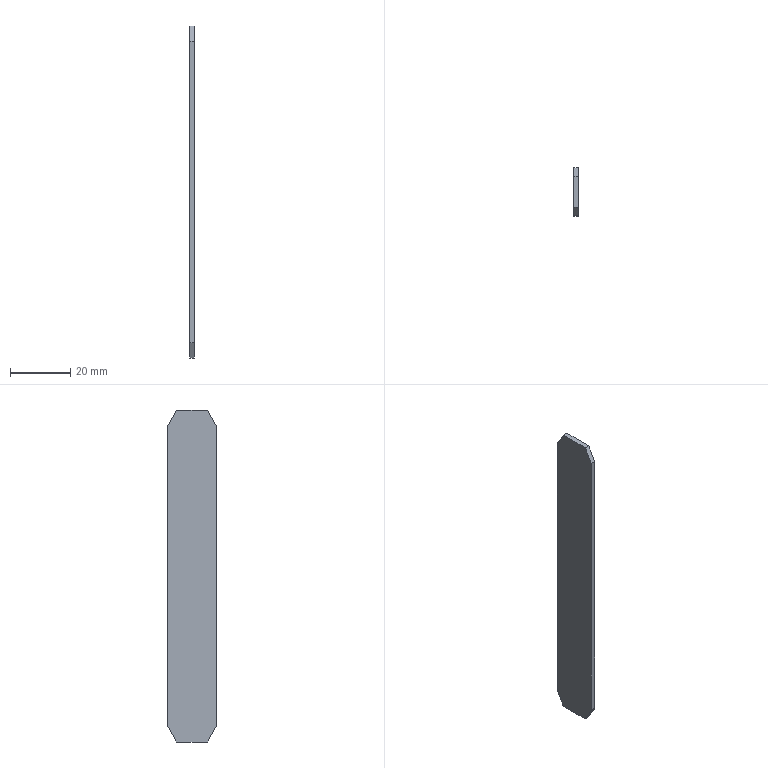Part | STEP file | 11-FG-B03111 | 1 solid | 10 faces | box 1.6 x 16 x 110 mm | volume 2770 mm3 | plane 10
STEP:
#1=CARTESIAN_POINT('',(0.8,-8.,105.));
#2=VERTEX_POINT('',#1);
#3=CARTESIAN_POINT('',(0.8,-8.,5.));
#4=VERTEX_POINT('',#3);
#5=CARTESIAN_POINT('',(0.8,-8.,110.));
#6=DIRECTION('',(0.,0.,-1.));
#7=VECTOR('',#6,1000.);
#8=LINE('',#5,#7);
#9=EDGE_CURVE('',#2,#4,#8,.T.);
#10=ORIENTED_EDGE('',*,*,#9,.T.);
#11=CARTESIAN_POINT('',(0.8,-5.113,0.));
#12=VERTEX_POINT('',#11);
#13=CARTESIAN_POINT('',(0.8,-8.,5.));
#14=DIRECTION('',(0.,0.5,-0.866));
#15=VECTOR('',#14,1000.);
#16=LINE('',#13,#15);
#17=EDGE_CURVE('',#4,#12,#16,.T.);
#18=ORIENTED_EDGE('',*,*,#17,.T.);
#19=CARTESIAN_POINT('',(0.8,5.113,0.));
#20=VERTEX_POINT('',#19);
#21=CARTESIAN_POINT('',(0.8,8.,0.));
#22=DIRECTION('',(0.,1.,0.));
#23=VECTOR('',#22,1000.);
#24=LINE('',#21,#23);
#25=EDGE_CURVE('',#12,#20,#24,.T.);
#26=ORIENTED_EDGE('',*,*,#25,.T.);
#27=CARTESIAN_POINT('',(0.8,8.,5.));
#28=VERTEX_POINT('',#27);
#29=CARTESIAN_POINT('',(0.8,8.,5.));
#30=DIRECTION('',(0.,0.5,0.866));
#31=VECTOR('',#30,1000.);
#32=LINE('',#29,#31);
#33=EDGE_CURVE('',#20,#28,#32,.T.);
#34=ORIENTED_EDGE('',*,*,#33,.T.);
#35=CARTESIAN_POINT('',(0.8,8.,105.));
#36=VERTEX_POINT('',#35);
#37=CARTESIAN_POINT('',(0.8,8.,110.));
#38=DIRECTION('',(0.,0.,-1.));
#39=VECTOR('',#38,1000.);
#40=LINE('',#37,#39);
#41=EDGE_CURVE('',#36,#28,#40,.T.);
#42=ORIENTED_EDGE('',*,*,#41,.F.);
#43=CARTESIAN_POINT('',(0.8,5.113,110.));
#44=VERTEX_POINT('',#43);
#45=CARTESIAN_POINT('',(0.8,5.113,110.));
#46=DIRECTION('',(0.,-0.5,0.866));
#47=VECTOR('',#46,1000.);
#48=LINE('',#45,#47);
#49=EDGE_CURVE('',#36,#44,#48,.T.);
#50=ORIENTED_EDGE('',*,*,#49,.T.);
#51=CARTESIAN_POINT('',(0.8,-5.113,110.));
#52=VERTEX_POINT('',#51);
#53=CARTESIAN_POINT('',(0.8,8.,110.));
#54=DIRECTION('',(0.,1.,0.));
#55=VECTOR('',#54,1000.);
#56=LINE('',#53,#55);
#57=EDGE_CURVE('',#52,#44,#56,.T.);
#58=ORIENTED_EDGE('',*,*,#57,.F.);
#59=CARTESIAN_POINT('',(0.8,-5.113,110.));
#60=DIRECTION('',(0.,-0.5,-0.866));
#61=VECTOR('',#60,1000.);
#62=LINE('',#59,#61);
#63=EDGE_CURVE('',#52,#2,#62,.T.);
#64=ORIENTED_EDGE('',*,*,#63,.T.);
#65=EDGE_LOOP('',(#10,#18,#26,#34,#42,#50,#58,#64));
#66=FACE_OUTER_BOUND('',#65,.T.);
#67=CARTESIAN_POINT('',(0.8,8.,110.));
#68=DIRECTION('',(-1.,0.,0.));
#69=DIRECTION('',(0.,-1.,0.));
#70=AXIS2_PLACEMENT_3D('',#67,#68,#69);
#71=PLANE('',#70);
#72=ADVANCED_FACE('',(#66),#71,.F.);
#73=ORIENTED_EDGE('',*,*,#41,.T.);
#74=CARTESIAN_POINT('',(-0.8,8.,5.));
#75=VERTEX_POINT('',#74);
#76=CARTESIAN_POINT('',(-0.8,8.,5.));
#77=DIRECTION('',(-1.,0.,0.));
#78=VECTOR('',#77,1000.);
#79=LINE('',#76,#78);
#80=EDGE_CURVE('',#28,#75,#79,.T.);
#81=ORIENTED_EDGE('',*,*,#80,.T.);
#82=CARTESIAN_POINT('',(-0.8,8.,105.));
#83=VERTEX_POINT('',#82);
#84=CARTESIAN_POINT('',(-0.8,8.,110.));
#85=DIRECTION('',(0.,0.,-1.));
#86=VECTOR('',#85,1000.);
#87=LINE('',#84,#86);
#88=EDGE_CURVE('',#83,#75,#87,.T.);
#89=ORIENTED_EDGE('',*,*,#88,.F.);
#90=CARTESIAN_POINT('',(0.8,8.,105.));
#91=DIRECTION('',(1.,0.,0.));
#92=VECTOR('',#91,1000.);
#93=LINE('',#90,#92);
#94=EDGE_CURVE('',#83,#36,#93,.T.);
#95=ORIENTED_EDGE('',*,*,#94,.T.);
#96=EDGE_LOOP('',(#73,#81,#89,#95));
#97=FACE_OUTER_BOUND('',#96,.T.);
#98=CARTESIAN_POINT('',(-0.8,8.,110.));
#99=DIRECTION('',(0.,-1.,0.));
#100=DIRECTION('',(0.,0.,-1.));
#101=AXIS2_PLACEMENT_3D('',#98,#99,#100);
#102=PLANE('',#101);
#103=ADVANCED_FACE('',(#97),#102,.F.);
#104=CARTESIAN_POINT('',(-0.8,5.113,0.));
#105=VERTEX_POINT('',#104);
#106=CARTESIAN_POINT('',(-0.8,-5.113,0.));
#107=VERTEX_POINT('',#106);
#108=CARTESIAN_POINT('',(-0.8,8.,0.));
#109=DIRECTION('',(0.,-1.,0.));
#110=VECTOR('',#109,1000.);
#111=LINE('',#108,#110);
#112=EDGE_CURVE('',#105,#107,#111,.T.);
#113=ORIENTED_EDGE('',*,*,#112,.T.);
#114=CARTESIAN_POINT('',(-0.8,-8.,5.));
#115=VERTEX_POINT('',#114);
#116=CARTESIAN_POINT('',(-0.8,-8.,5.));
#117=DIRECTION('',(0.,-0.5,0.866));
#118=VECTOR('',#117,1000.);
#119=LINE('',#116,#118);
#120=EDGE_CURVE('',#107,#115,#119,.T.);
#121=ORIENTED_EDGE('',*,*,#120,.T.);
#122=CARTESIAN_POINT('',(-0.8,-8.,105.));
#123=VERTEX_POINT('',#122);
#124=CARTESIAN_POINT('',(-0.8,-8.,110.));
#125=DIRECTION('',(0.,0.,-1.));
#126=VECTOR('',#125,1000.);
#127=LINE('',#124,#126);
#128=EDGE_CURVE('',#123,#115,#127,.T.);
#129=ORIENTED_EDGE('',*,*,#128,.F.);
#130=CARTESIAN_POINT('',(-0.8,-5.113,110.));
#131=VERTEX_POINT('',#130);
#132=CARTESIAN_POINT('',(-0.8,-5.113,110.));
#133=DIRECTION('',(0.,0.5,0.866));
#134=VECTOR('',#133,1000.);
#135=LINE('',#132,#134);
#136=EDGE_CURVE('',#123,#131,#135,.T.);
#137=ORIENTED_EDGE('',*,*,#136,.T.);
#138=CARTESIAN_POINT('',(-0.8,5.113,110.));
#139=VERTEX_POINT('',#138);
#140=CARTESIAN_POINT('',(-0.8,8.,110.));
#141=DIRECTION('',(0.,-1.,0.));
#142=VECTOR('',#141,1000.);
#143=LINE('',#140,#142);
#144=EDGE_CURVE('',#139,#131,#143,.T.);
#145=ORIENTED_EDGE('',*,*,#144,.F.);
#146=CARTESIAN_POINT('',(-0.8,5.113,110.));
#147=DIRECTION('',(0.,0.5,-0.866));
#148=VECTOR('',#147,1000.);
#149=LINE('',#146,#148);
#150=EDGE_CURVE('',#139,#83,#149,.T.);
#151=ORIENTED_EDGE('',*,*,#150,.T.);
#152=ORIENTED_EDGE('',*,*,#88,.T.);
#153=CARTESIAN_POINT('',(-0.8,8.,5.));
#154=DIRECTION('',(0.,-0.5,-0.866));
#155=VECTOR('',#154,1000.);
#156=LINE('',#153,#155);
#157=EDGE_CURVE('',#75,#105,#156,.T.);
#158=ORIENTED_EDGE('',*,*,#157,.T.);
#159=EDGE_LOOP('',(#113,#121,#129,#137,#145,#151,#152,#158));
#160=FACE_OUTER_BOUND('',#159,.T.);
#161=CARTESIAN_POINT('',(-0.8,8.,110.));
#162=DIRECTION('',(1.,0.,0.));
#163=DIRECTION('',(0.,1.,0.));
#164=AXIS2_PLACEMENT_3D('',#161,#162,#163);
#165=PLANE('',#164);
#166=ADVANCED_FACE('',(#160),#165,.F.);
#167=ORIENTED_EDGE('',*,*,#128,.T.);
#168=CARTESIAN_POINT('',(-0.8,-8.,5.));
#169=DIRECTION('',(1.,0.,0.));
#170=VECTOR('',#169,1000.);
#171=LINE('',#168,#170);
#172=EDGE_CURVE('',#115,#4,#171,.T.);
#173=ORIENTED_EDGE('',*,*,#172,.T.);
#174=ORIENTED_EDGE('',*,*,#9,.F.);
#175=CARTESIAN_POINT('',(-0.8,-8.,105.));
#176=DIRECTION('',(-1.,0.,0.));
#177=VECTOR('',#176,1000.);
#178=LINE('',#175,#177);
#179=EDGE_CURVE('',#2,#123,#178,.T.);
#180=ORIENTED_EDGE('',*,*,#179,.T.);
#181=EDGE_LOOP('',(#167,#173,#174,#180));
#182=FACE_OUTER_BOUND('',#181,.T.);
#183=CARTESIAN_POINT('',(-0.8,-8.,110.));
#184=DIRECTION('',(0.,1.,0.));
#185=DIRECTION('',(0.,0.,1.));
#186=AXIS2_PLACEMENT_3D('',#183,#184,#185);
#187=PLANE('',#186);
#188=ADVANCED_FACE('',(#182),#187,.F.);
#189=ORIENTED_EDGE('',*,*,#144,.T.);
#190=CARTESIAN_POINT('',(0.8,-5.113,110.));
#191=DIRECTION('',(1.,0.,0.));
#192=VECTOR('',#191,1000.);
#193=LINE('',#190,#192);
#194=EDGE_CURVE('',#131,#52,#193,.T.);
#195=ORIENTED_EDGE('',*,*,#194,.T.);
#196=ORIENTED_EDGE('',*,*,#57,.T.);
#197=CARTESIAN_POINT('',(-0.8,5.113,110.));
#198=DIRECTION('',(-1.,0.,0.));
#199=VECTOR('',#198,1000.);
#200=LINE('',#197,#199);
#201=EDGE_CURVE('',#44,#139,#200,.T.);
#202=ORIENTED_EDGE('',*,*,#201,.T.);
#203=EDGE_LOOP('',(#189,#195,#196,#202));
#204=FACE_OUTER_BOUND('',#203,.T.);
#205=CARTESIAN_POINT('',(0.,0.,110.));
#206=DIRECTION('',(0.,0.,1.));
#207=DIRECTION('',(1.,0.,0.));
#208=AXIS2_PLACEMENT_3D('',#205,#206,#207);
#209=PLANE('',#208);
#210=ADVANCED_FACE('',(#204),#209,.T.);
#211=ORIENTED_EDGE('',*,*,#25,.F.);
#212=CARTESIAN_POINT('',(0.,-5.113,0.));
#213=DIRECTION('',(-1.,0.,0.));
#214=VECTOR('',#213,1000.);
#215=LINE('',#212,#214);
#216=EDGE_CURVE('',#12,#107,#215,.T.);
#217=ORIENTED_EDGE('',*,*,#216,.T.);
#218=ORIENTED_EDGE('',*,*,#112,.F.);
#219=CARTESIAN_POINT('',(0.,5.113,0.));
#220=DIRECTION('',(1.,0.,0.));
#221=VECTOR('',#220,1000.);
#222=LINE('',#219,#221);
#223=EDGE_CURVE('',#105,#20,#222,.T.);
#224=ORIENTED_EDGE('',*,*,#223,.T.);
#225=EDGE_LOOP('',(#211,#217,#218,#224));
#226=FACE_OUTER_BOUND('',#225,.T.);
#227=CARTESIAN_POINT('',(0.,0.,0.));
#228=DIRECTION('',(0.,0.,1.));
#229=DIRECTION('',(1.,0.,0.));
#230=AXIS2_PLACEMENT_3D('',#227,#228,#229);
#231=PLANE('',#230);
#232=ADVANCED_FACE('',(#226),#231,.F.);
#233=ORIENTED_EDGE('',*,*,#136,.F.);
#234=ORIENTED_EDGE('',*,*,#179,.F.);
#235=ORIENTED_EDGE('',*,*,#63,.F.);
#236=ORIENTED_EDGE('',*,*,#194,.F.);
#237=EDGE_LOOP('',(#233,#234,#235,#236));
#238=FACE_OUTER_BOUND('',#237,.T.);
#239=CARTESIAN_POINT('',(0.,-5.113,110.));
#240=DIRECTION('',(0.,-0.866,0.5));
#241=DIRECTION('',(-1.,0.,0.));
#242=AXIS2_PLACEMENT_3D('',#239,#240,#241);
#243=PLANE('',#242);
#244=ADVANCED_FACE('',(#238),#243,.T.);
#245=ORIENTED_EDGE('',*,*,#49,.F.);
#246=ORIENTED_EDGE('',*,*,#94,.F.);
#247=ORIENTED_EDGE('',*,*,#150,.F.);
#248=ORIENTED_EDGE('',*,*,#201,.F.);
#249=EDGE_LOOP('',(#245,#246,#247,#248));
#250=FACE_OUTER_BOUND('',#249,.T.);
#251=CARTESIAN_POINT('',(0.,5.113,110.));
#252=DIRECTION('',(0.,0.866,0.5));
#253=DIRECTION('',(1.,0.,0.));
#254=AXIS2_PLACEMENT_3D('',#251,#252,#253);
#255=PLANE('',#254);
#256=ADVANCED_FACE('',(#250),#255,.T.);
#257=ORIENTED_EDGE('',*,*,#120,.F.);
#258=ORIENTED_EDGE('',*,*,#216,.F.);
#259=ORIENTED_EDGE('',*,*,#17,.F.);
#260=ORIENTED_EDGE('',*,*,#172,.F.);
#261=EDGE_LOOP('',(#257,#258,#259,#260));
#262=FACE_OUTER_BOUND('',#261,.T.);
#263=CARTESIAN_POINT('',(-0.8,-8.,5.));
#264=DIRECTION('',(0.,0.866,0.5));
#265=DIRECTION('',(1.,0.,0.));
#266=AXIS2_PLACEMENT_3D('',#263,#264,#265);
#267=PLANE('',#266);
#268=ADVANCED_FACE('',(#262),#267,.F.);
#269=ORIENTED_EDGE('',*,*,#33,.F.);
#270=ORIENTED_EDGE('',*,*,#223,.F.);
#271=ORIENTED_EDGE('',*,*,#157,.F.);
#272=ORIENTED_EDGE('',*,*,#80,.F.);
#273=EDGE_LOOP('',(#269,#270,#271,#272));
#274=FACE_OUTER_BOUND('',#273,.T.);
#275=CARTESIAN_POINT('',(-0.8,8.,5.));
#276=DIRECTION('',(0.,-0.866,0.5));
#277=DIRECTION('',(-1.,0.,0.));
#278=AXIS2_PLACEMENT_3D('',#275,#276,#277);
#279=PLANE('',#278);
#280=ADVANCED_FACE('',(#274),#279,.F.);
#281=CLOSED_SHELL('',(#72,#103,#166,#188,#210,#232,#244,#256,#268,#280));
#282=MANIFOLD_SOLID_BREP('',#281);
#283=CARTESIAN_POINT('',(0.,0.,0.));
#284=DIRECTION('',(0.,0.,1.));
#285=DIRECTION('',(1.,0.,0.));
#286=AXIS2_PLACEMENT_3D('',#283,#284,#285);
#287=(LENGTH_UNIT()NAMED_UNIT(*)SI_UNIT(.MILLI.,.METRE.));
#288=UNCERTAINTY_MEASURE_WITH_UNIT(LENGTH_MEASURE(0.00001),#287,'','');
#289=(NAMED_UNIT(*)PLANE_ANGLE_UNIT()SI_UNIT($,.RADIAN.));
#290=(NAMED_UNIT(*)SI_UNIT($,.STERADIAN.)SOLID_ANGLE_UNIT());
#291=(GEOMETRIC_REPRESENTATION_CONTEXT(3)GLOBAL_UNCERTAINTY_ASSIGNED_CONTEXT((#288))GLOBAL_UNIT_ASSIGNED_CONTEXT((#287,#289,#290))REPRESENTATION_CONTEXT('',''));
#292=ADVANCED_BREP_SHAPE_REPRESENTATION('',(#282,#286),#291);